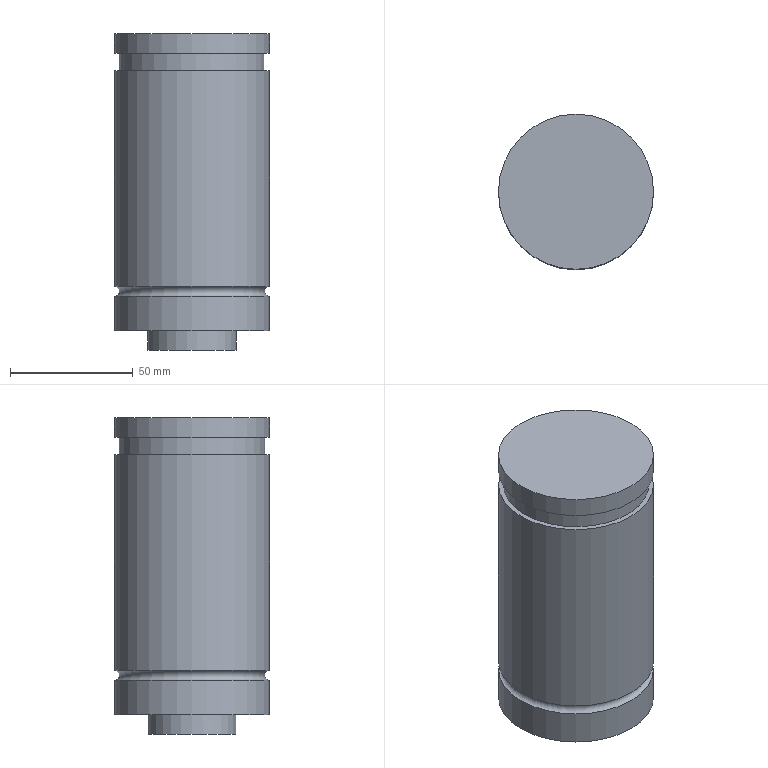Part | NX | features MAIN_BODY 2 | 1 solid | 11 faces | box 63.2 x 63.2 x 129 mm | volume 383823 mm3 | cylinder 5 | plane 5 | torus 1 | commonest cylinder face diameters 63.2 x3 36 x1 59.2 x1
STEP:
#1=CARTESIAN_POINT('',(1411.6,505.,370.));
#2=VERTEX_POINT('',#1);
#3=CARTESIAN_POINT('',(1380.,505.,370.));
#4=DIRECTION('',(0.,0.,1.));
#5=DIRECTION('',(1.,0.,0.));
#6=AXIS2_PLACEMENT_3D('',#3,#4,#5);
#7=CIRCLE('',#6,31.6);
#8=EDGE_CURVE('',#2,#2,#7,.F.);
#9=ORIENTED_EDGE('',*,*,#8,.T.);
#10=EDGE_LOOP('',(#9));
#11=FACE_BOUND('',#10,.T.);
#12=CARTESIAN_POINT('',(1411.6,505.,282.));
#13=VERTEX_POINT('',#12);
#14=CARTESIAN_POINT('',(1380.,505.,282.));
#15=DIRECTION('',(0.,0.,1.));
#16=DIRECTION('',(1.,0.,0.));
#17=AXIS2_PLACEMENT_3D('',#14,#15,#16);
#18=CIRCLE('',#17,31.6);
#19=EDGE_CURVE('',#13,#13,#18,.T.);
#20=ORIENTED_EDGE('',*,*,#19,.T.);
#21=EDGE_LOOP('',(#20));
#22=FACE_BOUND('',#21,.T.);
#23=CARTESIAN_POINT('',(1380.,505.,264.));
#24=DIRECTION('',(0.,0.,1.));
#25=DIRECTION('',(1.,0.,0.));
#26=AXIS2_PLACEMENT_3D('',#23,#24,#25);
#27=CYLINDRICAL_SURFACE('',#26,31.6);
#28=ADVANCED_FACE('',(#11,#22),#27,.T.);
#29=CARTESIAN_POINT('',(1348.4,505.,264.));
#30=VERTEX_POINT('',#29);
#31=CARTESIAN_POINT('',(1380.,505.,264.));
#32=DIRECTION('',(0.,0.,-1.));
#33=DIRECTION('',(-1.,0.,0.));
#34=AXIS2_PLACEMENT_3D('',#31,#32,#33);
#35=CIRCLE('',#34,31.6);
#36=EDGE_CURVE('',#30,#30,#35,.T.);
#37=ORIENTED_EDGE('',*,*,#36,.T.);
#38=EDGE_LOOP('',(#37));
#39=FACE_BOUND('',#38,.T.);
#40=CARTESIAN_POINT('',(1362.,505.,264.));
#41=VERTEX_POINT('',#40);
#42=CARTESIAN_POINT('',(1380.,505.,264.));
#43=DIRECTION('',(0.,0.,-1.));
#44=DIRECTION('',(-1.,0.,0.));
#45=AXIS2_PLACEMENT_3D('',#42,#43,#44);
#46=CIRCLE('',#45,18.);
#47=EDGE_CURVE('',#41,#41,#46,.T.);
#48=ORIENTED_EDGE('',*,*,#47,.F.);
#49=EDGE_LOOP('',(#48));
#50=FACE_BOUND('',#49,.T.);
#51=CARTESIAN_POINT('',(1380.,505.,264.));
#52=DIRECTION('',(0.,0.,-1.));
#53=DIRECTION('',(-1.,0.,0.));
#54=AXIS2_PLACEMENT_3D('',#51,#52,#53);
#55=PLANE('',#54);
#56=ADVANCED_FACE('',(#39,#50),#55,.T.);
#57=CARTESIAN_POINT('',(1411.6,505.,278.));
#58=VERTEX_POINT('',#57);
#59=CARTESIAN_POINT('',(1380.,505.,278.));
#60=DIRECTION('',(0.,0.,1.));
#61=DIRECTION('',(1.,0.,0.));
#62=AXIS2_PLACEMENT_3D('',#59,#60,#61);
#63=CIRCLE('',#62,31.6);
#64=EDGE_CURVE('',#58,#58,#63,.F.);
#65=ORIENTED_EDGE('',*,*,#64,.T.);
#66=EDGE_LOOP('',(#65));
#67=FACE_BOUND('',#66,.T.);
#68=ORIENTED_EDGE('',*,*,#36,.F.);
#69=EDGE_LOOP('',(#68));
#70=FACE_BOUND('',#69,.T.);
#71=CARTESIAN_POINT('',(1380.,505.,264.));
#72=DIRECTION('',(0.,0.,1.));
#73=DIRECTION('',(1.,0.,0.));
#74=AXIS2_PLACEMENT_3D('',#71,#72,#73);
#75=CYLINDRICAL_SURFACE('',#74,31.6);
#76=ADVANCED_FACE('',(#67,#70),#75,.T.);
#77=ORIENTED_EDGE('',*,*,#47,.T.);
#78=EDGE_LOOP('',(#77));
#79=FACE_BOUND('',#78,.T.);
#80=CARTESIAN_POINT('',(1362.,505.,256.));
#81=VERTEX_POINT('',#80);
#82=CARTESIAN_POINT('',(1380.,505.,256.));
#83=DIRECTION('',(0.,0.,-1.));
#84=DIRECTION('',(-1.,0.,0.));
#85=AXIS2_PLACEMENT_3D('',#82,#83,#84);
#86=CIRCLE('',#85,18.);
#87=EDGE_CURVE('',#81,#81,#86,.T.);
#88=ORIENTED_EDGE('',*,*,#87,.F.);
#89=EDGE_LOOP('',(#88));
#90=FACE_BOUND('',#89,.T.);
#91=CARTESIAN_POINT('',(1380.,505.,261.));
#92=DIRECTION('',(0.,0.,1.));
#93=DIRECTION('',(1.,0.,0.));
#94=AXIS2_PLACEMENT_3D('',#91,#92,#93);
#95=CYLINDRICAL_SURFACE('',#94,18.);
#96=ADVANCED_FACE('',(#79,#90),#95,.T.);
#97=ORIENTED_EDGE('',*,*,#64,.F.);
#98=EDGE_LOOP('',(#97));
#99=FACE_BOUND('',#98,.T.);
#100=ORIENTED_EDGE('',*,*,#19,.F.);
#101=EDGE_LOOP('',(#100));
#102=FACE_BOUND('',#101,.T.);
#103=CARTESIAN_POINT('',(1380.,505.,280.));
#104=DIRECTION('',(0.,0.,1.));
#105=DIRECTION('',(1.,0.,0.));
#106=AXIS2_PLACEMENT_3D('',#103,#104,#105);
#107=TOROIDAL_SURFACE('',#106,31.6,2.);
#108=ADVANCED_FACE('',(#99,#102),#107,.F.);
#109=CARTESIAN_POINT('',(1350.4,505.,370.));
#110=VERTEX_POINT('',#109);
#111=CARTESIAN_POINT('',(1380.,505.,370.));
#112=DIRECTION('',(0.,0.,-1.));
#113=DIRECTION('',(-1.,0.,0.));
#114=AXIS2_PLACEMENT_3D('',#111,#112,#113);
#115=CIRCLE('',#114,29.6);
#116=EDGE_CURVE('',#110,#110,#115,.T.);
#117=ORIENTED_EDGE('',*,*,#116,.T.);
#118=EDGE_LOOP('',(#117));
#119=FACE_BOUND('',#118,.T.);
#120=ORIENTED_EDGE('',*,*,#8,.F.);
#121=EDGE_LOOP('',(#120));
#122=FACE_BOUND('',#121,.T.);
#123=CARTESIAN_POINT('',(1380.,505.,370.));
#124=DIRECTION('',(0.,0.,1.));
#125=DIRECTION('',(1.,0.,0.));
#126=AXIS2_PLACEMENT_3D('',#123,#124,#125);
#127=PLANE('',#126);
#128=ADVANCED_FACE('',(#119,#122),#127,.T.);
#129=CARTESIAN_POINT('',(1350.4,505.,377.));
#130=VERTEX_POINT('',#129);
#131=CARTESIAN_POINT('',(1380.,505.,377.));
#132=DIRECTION('',(0.,0.,-1.));
#133=DIRECTION('',(-1.,0.,0.));
#134=AXIS2_PLACEMENT_3D('',#131,#132,#133);
#135=CIRCLE('',#134,29.6);
#136=EDGE_CURVE('',#130,#130,#135,.T.);
#137=ORIENTED_EDGE('',*,*,#136,.F.);
#138=EDGE_LOOP('',(#137));
#139=FACE_BOUND('',#138,.T.);
#140=CARTESIAN_POINT('',(1411.6,505.,377.));
#141=VERTEX_POINT('',#140);
#142=CARTESIAN_POINT('',(1380.,505.,377.));
#143=DIRECTION('',(0.,0.,1.));
#144=DIRECTION('',(1.,0.,0.));
#145=AXIS2_PLACEMENT_3D('',#142,#143,#144);
#146=CIRCLE('',#145,31.6);
#147=EDGE_CURVE('',#141,#141,#146,.T.);
#148=ORIENTED_EDGE('',*,*,#147,.F.);
#149=EDGE_LOOP('',(#148));
#150=FACE_BOUND('',#149,.T.);
#151=CARTESIAN_POINT('',(1380.,505.,377.));
#152=DIRECTION('',(0.,0.,1.));
#153=DIRECTION('',(1.,0.,0.));
#154=AXIS2_PLACEMENT_3D('',#151,#152,#153);
#155=PLANE('',#154);
#156=ADVANCED_FACE('',(#139,#150),#155,.F.);
#157=ORIENTED_EDGE('',*,*,#116,.F.);
#158=EDGE_LOOP('',(#157));
#159=FACE_BOUND('',#158,.T.);
#160=ORIENTED_EDGE('',*,*,#136,.T.);
#161=EDGE_LOOP('',(#160));
#162=FACE_BOUND('',#161,.T.);
#163=CARTESIAN_POINT('',(1380.,505.,377.));
#164=DIRECTION('',(0.,0.,-1.));
#165=DIRECTION('',(-1.,0.,0.));
#166=AXIS2_PLACEMENT_3D('',#163,#164,#165);
#167=CYLINDRICAL_SURFACE('',#166,29.6);
#168=ADVANCED_FACE('',(#159,#162),#167,.T.);
#169=CARTESIAN_POINT('',(1348.4,505.,385.));
#170=VERTEX_POINT('',#169);
#171=CARTESIAN_POINT('',(1380.,505.,385.));
#172=DIRECTION('',(0.,0.,-1.));
#173=DIRECTION('',(-1.,0.,0.));
#174=AXIS2_PLACEMENT_3D('',#171,#172,#173);
#175=CIRCLE('',#174,31.6);
#176=EDGE_CURVE('',#170,#170,#175,.T.);
#177=ORIENTED_EDGE('',*,*,#176,.F.);
#178=EDGE_LOOP('',(#177));
#179=FACE_BOUND('',#178,.T.);
#180=CARTESIAN_POINT('',(1380.,505.,385.));
#181=DIRECTION('',(0.,0.,-1.));
#182=DIRECTION('',(-1.,0.,0.));
#183=AXIS2_PLACEMENT_3D('',#180,#181,#182);
#184=PLANE('',#183);
#185=ADVANCED_FACE('',(#179),#184,.F.);
#186=ORIENTED_EDGE('',*,*,#147,.T.);
#187=EDGE_LOOP('',(#186));
#188=FACE_BOUND('',#187,.T.);
#189=ORIENTED_EDGE('',*,*,#176,.T.);
#190=EDGE_LOOP('',(#189));
#191=FACE_BOUND('',#190,.T.);
#192=CARTESIAN_POINT('',(1380.,505.,264.));
#193=DIRECTION('',(0.,0.,1.));
#194=DIRECTION('',(1.,0.,0.));
#195=AXIS2_PLACEMENT_3D('',#192,#193,#194);
#196=CYLINDRICAL_SURFACE('',#195,31.6);
#197=ADVANCED_FACE('',(#188,#191),#196,.T.);
#198=ORIENTED_EDGE('',*,*,#87,.T.);
#199=EDGE_LOOP('',(#198));
#200=FACE_BOUND('',#199,.T.);
#201=CARTESIAN_POINT('',(1380.,505.,256.));
#202=DIRECTION('',(0.,0.,-1.));
#203=DIRECTION('',(-1.,0.,0.));
#204=AXIS2_PLACEMENT_3D('',#201,#202,#203);
#205=PLANE('',#204);
#206=ADVANCED_FACE('',(#200),#205,.T.);
#207=CLOSED_SHELL('',(#28,#56,#76,#96,#108,#128,#156,#168,#185,#197,#206));
#208=MANIFOLD_SOLID_BREP('',#207);
#209=(LENGTH_UNIT()NAMED_UNIT(*)SI_UNIT(.MILLI.,.METRE.));
#210=UNCERTAINTY_MEASURE_WITH_UNIT(LENGTH_MEASURE(0.00001),#209,'','');
#211=(NAMED_UNIT(*)PLANE_ANGLE_UNIT()SI_UNIT($,.RADIAN.));
#212=(NAMED_UNIT(*)SI_UNIT($,.STERADIAN.)SOLID_ANGLE_UNIT());
#213=(GEOMETRIC_REPRESENTATION_CONTEXT(3)GLOBAL_UNCERTAINTY_ASSIGNED_CONTEXT((#210))GLOBAL_UNIT_ASSIGNED_CONTEXT((#209,#211,#212))REPRESENTATION_CONTEXT('',''));
#214=ADVANCED_BREP_SHAPE_REPRESENTATION('',(#208),#213);